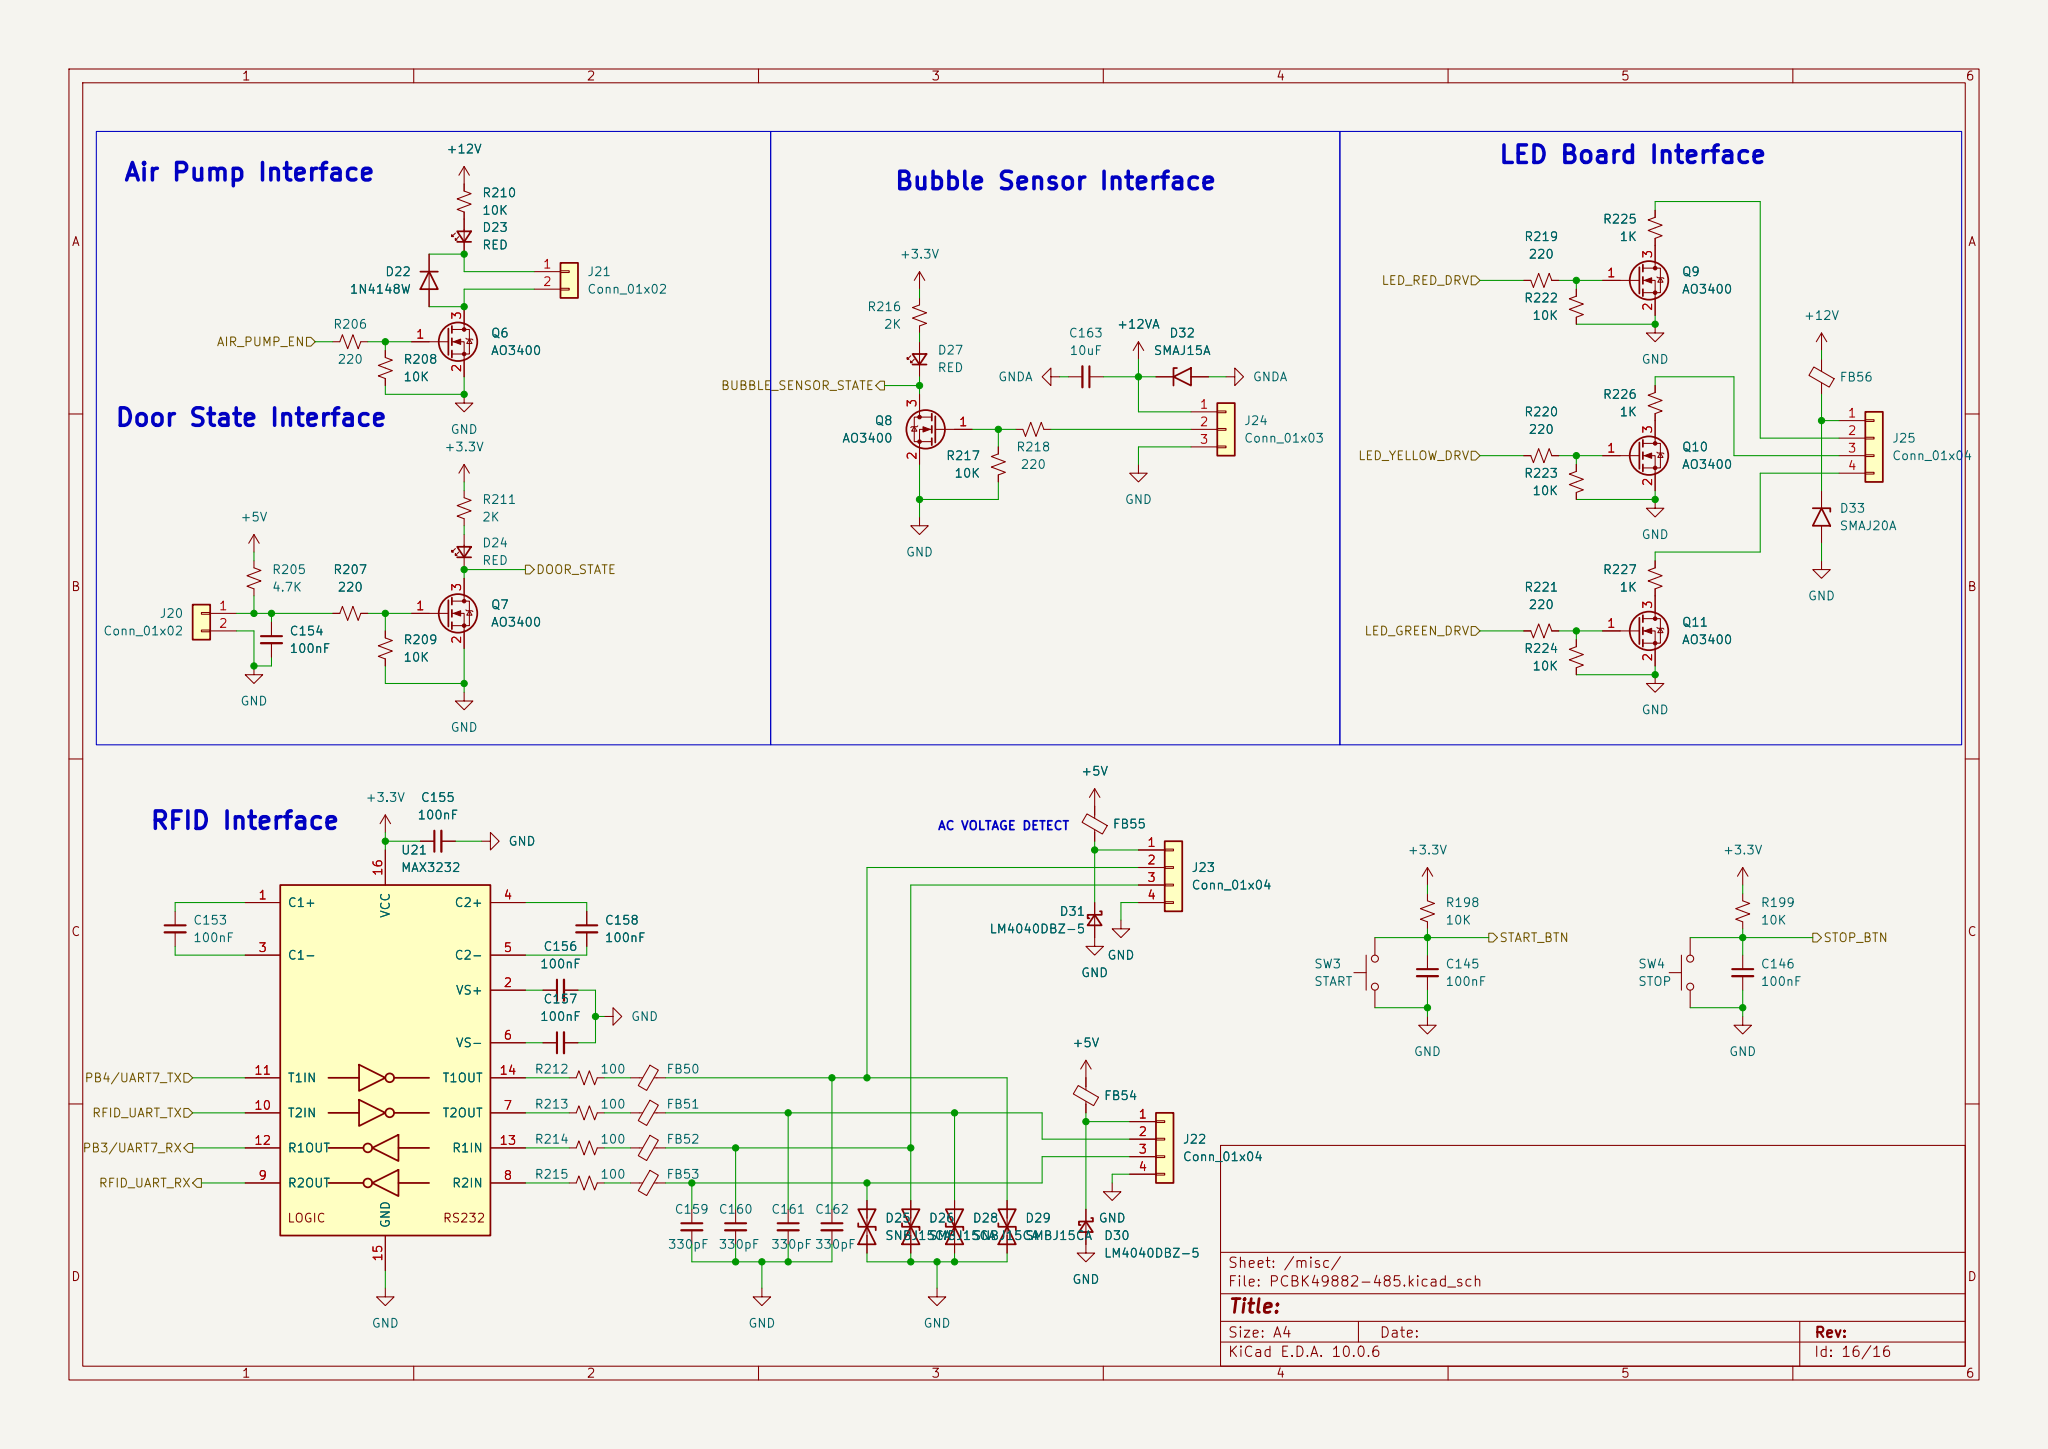Circuit board | KiCad | 536 parts | 438 nets | one sheet of the schematic
Parts on this sheet (reference | value | footprint):
C145 | 100nF | Capacitor_SMD:C_0603_1608Metric
C146 | 100nF | Capacitor_SMD:C_0603_1608Metric
C153
C154
C155
C156
C157
C158
C159
C160
C161
C162
C163 | 10uF | Capacitor_SMD:C_1210_3225Metric
D22 | 1N4148W | Diode_SMD:D_SOD-123
D23 | RED | LED_SMD:LED_0603_1608Metric
D24 | RED | LED_SMD:LED_0603_1608Metric
D25 | SNBJ15CA | Diode_SMD:D_SMB
D26 | SMBJ15CA | Diode_SMD:D_SMB
D27 | RED | LED_SMD:LED_0603_1608Metric
D28 | SNBJ15CA | Diode_SMD:D_SMB
D29 | SMBJ15CA | Diode_SMD:D_SMB
D30 | LM4040DBZ-5 | Package_TO_SOT_SMD:SOT-23
D31 | LM4040DBZ-5 | Package_TO_SOT_SMD:SOT-23
D32 | SMAJ15A | Diode_SMD:D_SMA
D33 | SMAJ20A | Diode_SMD:D_SMA
FB50
FB51
FB52
FB53
FB54
FB55
FB56
J20
J21
J22 | Conn_01x04 | Connector_Molex:Molex_MicroClasp_55932-0430_1x04_P2.00mm_Vertical
J23 | Conn_01x04 | Connector_Molex:Molex_MicroClasp_55932-0430_1x04_P2.00mm_Vertical
J24 | Conn_01x03 | Connector_Molex:Molex_MicroClasp_55932-0330_1x03_P2.00mm_Vertical
J25 | Conn_01x04 | Connector_Molex:Molex_MicroClasp_55932-0430_1x04_P2.00mm_Vertical
Q10
Q11
Q8
Q9
R198
R205 | 4.7K | Resistor_SMD:R_0603_1608Metric
R206 | 220 | Resistor_SMD:R_0603_1608Metric
R207 | 220 | Resistor_SMD:R_0603_1608Metric
R208
R209
R210
R211 | 2K | Resistor_SMD:R_0603_1608Metric
R212
R213
R214
R215
R216 | 2K | Resistor_SMD:R_0603_1608Metric
R217 | 10K | Resistor_SMD:R_0603_1608Metric
R218
R219
R220
R221
R222
R223
R224
R225
R226
R227
SW3 | START | Button_Switch_SMD:SW_Push_1P1T_NO_6x6mm_H9.5mm
SW4 | STOP | Button_Switch_SMD:SW_Push_1P1T_NO_6x6mm_H9.5mm
U21 | MAX3232 | Package_SO:SOIC-16_3.9x9.9mm_P1.27mm
Nets of these parts (net: part-pin ...):
+3.3V: C155-1 R198-1 R211-2 R216-2 U21-16
+5V: FB54-2 FB55-2 R205-1
+12V: FB56-2 R210-2
+12VA: C163-1 D32-1 J24-1
/core_board_b2b/PA15{slash}STOP_BTN: C146-1 SW4-2
/core_board_b2b/PB3{slash}UART7_RX: U21-12
/core_board_b2b/PB4{slash}UART7_TX: U21-11
/core_board_b2b/PC13{slash}LED_RED_DRV: R219-2
/core_board_b2b/PD5{slash}USART2_TX: U21-10
/core_board_b2b/PD6{slash}USART2_RX: U21-9
/core_board_b2b/PD7{slash}START_BTN: C145-1 R198-2 SW3-2
/core_board_b2b/PD11{slash}LED_YELLOW_DRV: R220-2
/core_board_b2b/PG3{slash}LED_GREEN_DRV: R221-2
/core_board_b2b/PH6{slash}DOOR_STATE: D24-1
/core_board_b2b/PI8{slash}AIR_PUMP_EN: R206-1
/core_board_b2b/PI11{slash}BUBBLE_SENSOR_STATE: D27-1 Q8-3
GND: C145-2 C146-2 C154-2 C155-2 C156-2 C157-2 C159-2 C160-2 C161-2 C162-2 D25-1 D26-1 D28-1 D29-1 D30-2 D31-2 D33-2 J20-2 J22-4 J23-4 J24-3 Q8-2 Q9-2 Q10-2 Q11-2 R208-1 R209-1 R217-1 R222-2 R223-2 R224-2 SW3-1 SW4-1 U21-15
GNDA: C163-2 D32-2
Net-(D22-A): D22-2 J21-2
Net-(D22-K): D22-1 D23-1 J21-1
Net-(D23-A): D23-2 R210-1
Net-(D24-A): D24-2 R211-1
Net-(D25-A2): C159-1 D25-2 FB53-1 J22-3
Net-(D26-A2): C160-1 D26-2 FB52-1 J23-3
Net-(D27-A): D27-2 R216-1
Net-(D28-A2): C161-1 D28-2 FB51-1 J22-2
Net-(D29-A2): C162-1 D29-2 FB50-1 J23-2
Net-(D30-K): D30-1 FB54-1 J22-1
Net-(D31-K): D31-1 FB55-1 J23-1
Net-(D33-A1): D33-1 FB56-1 J25-1
Net-(FB50-Pad2): FB50-2 R212-2
Net-(FB51-Pad2): FB51-2 R213-2
Net-(FB52-Pad2): FB52-2 R214-2
Net-(FB53-Pad2): FB53-2 R215-2
Net-(J20-Pin_1): C154-1 J20-1 R205-2 R207-1
Net-(J24-Pin_2): J24-2 R218-1
Net-(J25-Pin_2): J25-2 R225-1
Net-(J25-Pin_3): J25-3 R226-1
Net-(J25-Pin_4): J25-4 R227-1
Net-(Q6-G): R206-2 R208-2
Net-(Q7-G): R207-2 R209-2
Net-(Q8-G): Q8-1 R217-2 R218-2
Net-(Q9-D): Q9-3 R225-2
Net-(Q9-G): Q9-1 R219-1 R222-1
Net-(Q10-D): Q10-3 R226-2
Net-(Q10-G): Q10-1 R220-1 R223-1
Net-(Q11-D): Q11-3 R227-2
Net-(Q11-G): Q11-1 R221-1 R224-1
Net-(U21-C1+): C153-1 U21-1
Net-(U21-C1-): C153-2 U21-3
Net-(U21-C2+): C158-1 U21-4
Net-(U21-C2-): C158-2 U21-5
Net-(U21-R1IN): R214-1 U21-13
Net-(U21-R2IN): R215-1 U21-8
Net-(U21-T1OUT): R212-1 U21-14
Net-(U21-T2OUT): R213-1 U21-7
Net-(U21-VS+): C156-1 U21-2
Net-(U21-VS-): C157-1 U21-6